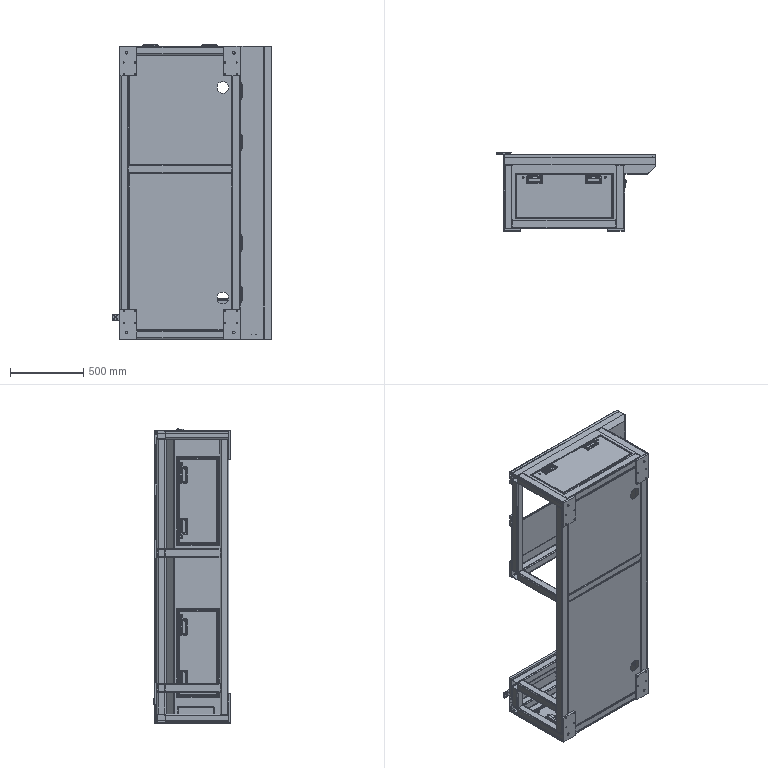Part | NX | features BREP 44 | 57 solids | 3099 faces | volume 27822882 mm3 | plane 1535 | cylinder 1187 | spline 152 | torus 130 | cone 95 | commonest cylinder face diameters 7 x139 8 x131 4 x124 6 x84 6.8 x77 16 x77